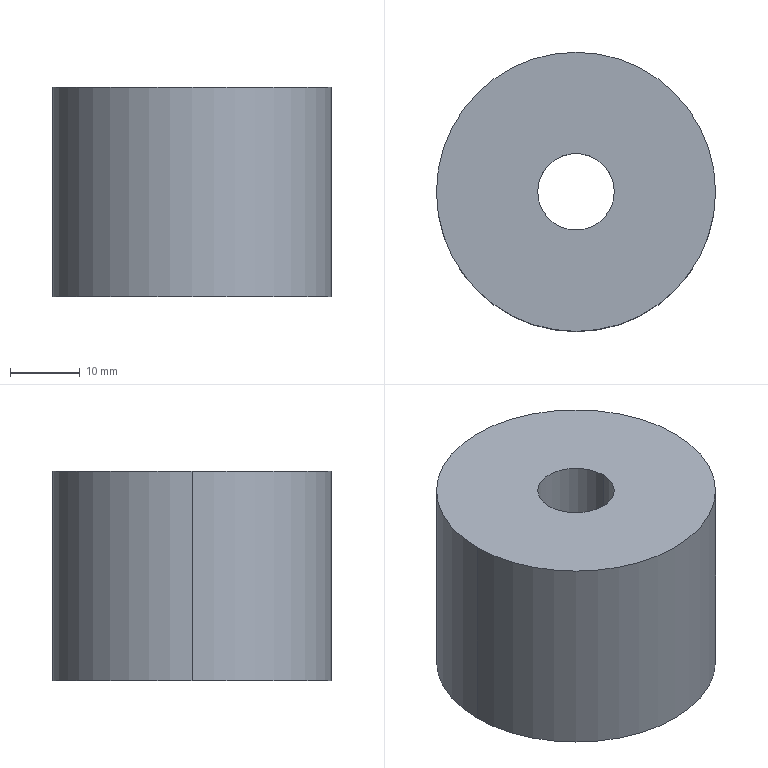Part | STEP file | X77-03029 | 1 solid | 9 faces | box 40 x 40 x 30 mm | volume 33094 mm3 | cylinder 6 | plane 3 | commonest cylinder face diameters 11 x2 18 x2 40 x2
STEP:
#1=CARTESIAN_POINT('',(9.,0.,11.));
#2=VERTEX_POINT('',#1);
#3=CARTESIAN_POINT('',(-9.,0.,11.));
#4=VERTEX_POINT('',#3);
#5=CARTESIAN_POINT('',(0.,0.,11.));
#6=DIRECTION('',(0.,0.,-1.));
#7=DIRECTION('',(-1.,0.,0.));
#8=AXIS2_PLACEMENT_3D('',#5,#6,#7);
#9=CIRCLE('',#8,9.);
#10=EDGE_CURVE('',#2,#4,#9,.T.);
#11=ORIENTED_EDGE('',*,*,#10,.F.);
#12=CARTESIAN_POINT('',(9.,0.,0.));
#13=VERTEX_POINT('',#12);
#14=CARTESIAN_POINT('',(9.,0.,0.));
#15=DIRECTION('',(0.,0.,-1.));
#16=VECTOR('',#15,1000.);
#17=LINE('',#14,#16);
#18=EDGE_CURVE('',#2,#13,#17,.T.);
#19=ORIENTED_EDGE('',*,*,#18,.T.);
#20=CARTESIAN_POINT('',(-9.,0.,0.));
#21=VERTEX_POINT('',#20);
#22=CARTESIAN_POINT('',(0.,0.,0.));
#23=DIRECTION('',(0.,0.,-1.));
#24=DIRECTION('',(-1.,0.,0.));
#25=AXIS2_PLACEMENT_3D('',#22,#23,#24);
#26=CIRCLE('',#25,9.);
#27=EDGE_CURVE('',#13,#21,#26,.T.);
#28=ORIENTED_EDGE('',*,*,#27,.T.);
#29=CARTESIAN_POINT('',(-9.,0.,0.));
#30=DIRECTION('',(0.,0.,-1.));
#31=VECTOR('',#30,1000.);
#32=LINE('',#29,#31);
#33=EDGE_CURVE('',#4,#21,#32,.T.);
#34=ORIENTED_EDGE('',*,*,#33,.F.);
#35=EDGE_LOOP('',(#11,#19,#28,#34));
#36=FACE_OUTER_BOUND('',#35,.T.);
#37=CARTESIAN_POINT('',(0.,0.,0.));
#38=DIRECTION('',(0.,0.,-1.));
#39=DIRECTION('',(-1.,0.,0.));
#40=AXIS2_PLACEMENT_3D('',#37,#38,#39);
#41=CYLINDRICAL_SURFACE('',#40,9.);
#42=ADVANCED_FACE('',(#36),#41,.F.);
#43=CARTESIAN_POINT('',(5.5,0.,30.));
#44=VERTEX_POINT('',#43);
#45=CARTESIAN_POINT('',(-5.5,0.,30.));
#46=VERTEX_POINT('',#45);
#47=CARTESIAN_POINT('',(0.,0.,30.));
#48=DIRECTION('',(0.,0.,-1.));
#49=DIRECTION('',(-1.,0.,0.));
#50=AXIS2_PLACEMENT_3D('',#47,#48,#49);
#51=CIRCLE('',#50,5.5);
#52=EDGE_CURVE('',#44,#46,#51,.T.);
#53=ORIENTED_EDGE('',*,*,#52,.F.);
#54=CARTESIAN_POINT('',(5.5,0.,11.));
#55=VERTEX_POINT('',#54);
#56=CARTESIAN_POINT('',(5.5,0.,0.));
#57=DIRECTION('',(0.,0.,-1.));
#58=VECTOR('',#57,1000.);
#59=LINE('',#56,#58);
#60=EDGE_CURVE('',#44,#55,#59,.T.);
#61=ORIENTED_EDGE('',*,*,#60,.T.);
#62=CARTESIAN_POINT('',(-5.5,0.,11.));
#63=VERTEX_POINT('',#62);
#64=CARTESIAN_POINT('',(0.,0.,11.));
#65=DIRECTION('',(0.,0.,-1.));
#66=DIRECTION('',(-1.,0.,0.));
#67=AXIS2_PLACEMENT_3D('',#64,#65,#66);
#68=CIRCLE('',#67,5.5);
#69=EDGE_CURVE('',#55,#63,#68,.T.);
#70=ORIENTED_EDGE('',*,*,#69,.T.);
#71=CARTESIAN_POINT('',(-5.5,0.,0.));
#72=DIRECTION('',(0.,0.,-1.));
#73=VECTOR('',#72,1000.);
#74=LINE('',#71,#73);
#75=EDGE_CURVE('',#46,#63,#74,.T.);
#76=ORIENTED_EDGE('',*,*,#75,.F.);
#77=EDGE_LOOP('',(#53,#61,#70,#76));
#78=FACE_OUTER_BOUND('',#77,.T.);
#79=CARTESIAN_POINT('',(0.,0.,0.));
#80=DIRECTION('',(0.,0.,-1.));
#81=DIRECTION('',(-1.,0.,0.));
#82=AXIS2_PLACEMENT_3D('',#79,#80,#81);
#83=CYLINDRICAL_SURFACE('',#82,5.5);
#84=ADVANCED_FACE('',(#78),#83,.F.);
#85=CARTESIAN_POINT('',(20.,0.,30.));
#86=VERTEX_POINT('',#85);
#87=CARTESIAN_POINT('',(-20.,0.,30.));
#88=VERTEX_POINT('',#87);
#89=CARTESIAN_POINT('',(0.,0.,30.));
#90=DIRECTION('',(0.,0.,1.));
#91=DIRECTION('',(1.,0.,0.));
#92=AXIS2_PLACEMENT_3D('',#89,#90,#91);
#93=CIRCLE('',#92,20.);
#94=EDGE_CURVE('',#86,#88,#93,.T.);
#95=ORIENTED_EDGE('',*,*,#94,.F.);
#96=CARTESIAN_POINT('',(20.,0.,0.));
#97=VERTEX_POINT('',#96);
#98=CARTESIAN_POINT('',(20.,0.,30.));
#99=DIRECTION('',(0.,0.,-1.));
#100=VECTOR('',#99,1000.);
#101=LINE('',#98,#100);
#102=EDGE_CURVE('',#86,#97,#101,.T.);
#103=ORIENTED_EDGE('',*,*,#102,.T.);
#104=CARTESIAN_POINT('',(-20.,0.,0.));
#105=VERTEX_POINT('',#104);
#106=CARTESIAN_POINT('',(0.,0.,0.));
#107=DIRECTION('',(0.,0.,1.));
#108=DIRECTION('',(1.,0.,0.));
#109=AXIS2_PLACEMENT_3D('',#106,#107,#108);
#110=CIRCLE('',#109,20.);
#111=EDGE_CURVE('',#97,#105,#110,.T.);
#112=ORIENTED_EDGE('',*,*,#111,.T.);
#113=CARTESIAN_POINT('',(-20.,0.,30.));
#114=DIRECTION('',(0.,0.,-1.));
#115=VECTOR('',#114,1000.);
#116=LINE('',#113,#115);
#117=EDGE_CURVE('',#88,#105,#116,.T.);
#118=ORIENTED_EDGE('',*,*,#117,.F.);
#119=EDGE_LOOP('',(#95,#103,#112,#118));
#120=FACE_OUTER_BOUND('',#119,.T.);
#121=CARTESIAN_POINT('',(0.,0.,30.));
#122=DIRECTION('',(0.,0.,-1.));
#123=DIRECTION('',(-1.,0.,0.));
#124=AXIS2_PLACEMENT_3D('',#121,#122,#123);
#125=CYLINDRICAL_SURFACE('',#124,20.);
#126=ADVANCED_FACE('',(#120),#125,.T.);
#127=ORIENTED_EDGE('',*,*,#102,.F.);
#128=CARTESIAN_POINT('',(0.,0.,30.));
#129=DIRECTION('',(0.,0.,1.));
#130=DIRECTION('',(1.,0.,0.));
#131=AXIS2_PLACEMENT_3D('',#128,#129,#130);
#132=CIRCLE('',#131,20.);
#133=EDGE_CURVE('',#88,#86,#132,.T.);
#134=ORIENTED_EDGE('',*,*,#133,.F.);
#135=ORIENTED_EDGE('',*,*,#117,.T.);
#136=CARTESIAN_POINT('',(0.,0.,0.));
#137=DIRECTION('',(0.,0.,1.));
#138=DIRECTION('',(1.,0.,0.));
#139=AXIS2_PLACEMENT_3D('',#136,#137,#138);
#140=CIRCLE('',#139,20.);
#141=EDGE_CURVE('',#105,#97,#140,.T.);
#142=ORIENTED_EDGE('',*,*,#141,.T.);
#143=EDGE_LOOP('',(#127,#134,#135,#142));
#144=FACE_OUTER_BOUND('',#143,.T.);
#145=CARTESIAN_POINT('',(0.,0.,30.));
#146=DIRECTION('',(0.,0.,-1.));
#147=DIRECTION('',(-1.,0.,0.));
#148=AXIS2_PLACEMENT_3D('',#145,#146,#147);
#149=CYLINDRICAL_SURFACE('',#148,20.);
#150=ADVANCED_FACE('',(#144),#149,.T.);
#151=CARTESIAN_POINT('',(0.,0.,30.));
#152=DIRECTION('',(0.,0.,-1.));
#153=DIRECTION('',(-1.,0.,0.));
#154=AXIS2_PLACEMENT_3D('',#151,#152,#153);
#155=CIRCLE('',#154,5.5);
#156=EDGE_CURVE('',#46,#44,#155,.T.);
#157=ORIENTED_EDGE('',*,*,#156,.T.);
#158=ORIENTED_EDGE('',*,*,#52,.T.);
#159=EDGE_LOOP('',(#157,#158));
#160=FACE_BOUND('',#159,.T.);
#161=ORIENTED_EDGE('',*,*,#133,.T.);
#162=ORIENTED_EDGE('',*,*,#94,.T.);
#163=EDGE_LOOP('',(#161,#162));
#164=FACE_OUTER_BOUND('',#163,.T.);
#165=CARTESIAN_POINT('',(0.,0.,30.));
#166=DIRECTION('',(0.,0.,1.));
#167=DIRECTION('',(1.,0.,0.));
#168=AXIS2_PLACEMENT_3D('',#165,#166,#167);
#169=PLANE('',#168);
#170=ADVANCED_FACE('',(#160,#164),#169,.T.);
#171=CARTESIAN_POINT('',(0.,0.,0.));
#172=DIRECTION('',(0.,0.,-1.));
#173=DIRECTION('',(-1.,0.,0.));
#174=AXIS2_PLACEMENT_3D('',#171,#172,#173);
#175=CIRCLE('',#174,9.);
#176=EDGE_CURVE('',#21,#13,#175,.T.);
#177=ORIENTED_EDGE('',*,*,#176,.F.);
#178=ORIENTED_EDGE('',*,*,#27,.F.);
#179=EDGE_LOOP('',(#177,#178));
#180=FACE_BOUND('',#179,.T.);
#181=ORIENTED_EDGE('',*,*,#141,.F.);
#182=ORIENTED_EDGE('',*,*,#111,.F.);
#183=EDGE_LOOP('',(#181,#182));
#184=FACE_OUTER_BOUND('',#183,.T.);
#185=CARTESIAN_POINT('',(0.,0.,0.));
#186=DIRECTION('',(0.,0.,1.));
#187=DIRECTION('',(1.,0.,0.));
#188=AXIS2_PLACEMENT_3D('',#185,#186,#187);
#189=PLANE('',#188);
#190=ADVANCED_FACE('',(#180,#184),#189,.F.);
#191=ORIENTED_EDGE('',*,*,#60,.F.);
#192=ORIENTED_EDGE('',*,*,#156,.F.);
#193=ORIENTED_EDGE('',*,*,#75,.T.);
#194=CARTESIAN_POINT('',(0.,0.,11.));
#195=DIRECTION('',(0.,0.,-1.));
#196=DIRECTION('',(-1.,0.,0.));
#197=AXIS2_PLACEMENT_3D('',#194,#195,#196);
#198=CIRCLE('',#197,5.5);
#199=EDGE_CURVE('',#63,#55,#198,.T.);
#200=ORIENTED_EDGE('',*,*,#199,.T.);
#201=EDGE_LOOP('',(#191,#192,#193,#200));
#202=FACE_OUTER_BOUND('',#201,.T.);
#203=CARTESIAN_POINT('',(0.,0.,0.));
#204=DIRECTION('',(0.,0.,-1.));
#205=DIRECTION('',(-1.,0.,0.));
#206=AXIS2_PLACEMENT_3D('',#203,#204,#205);
#207=CYLINDRICAL_SURFACE('',#206,5.5);
#208=ADVANCED_FACE('',(#202),#207,.F.);
#209=ORIENTED_EDGE('',*,*,#199,.F.);
#210=ORIENTED_EDGE('',*,*,#69,.F.);
#211=EDGE_LOOP('',(#209,#210));
#212=FACE_BOUND('',#211,.T.);
#213=CARTESIAN_POINT('',(0.,0.,11.));
#214=DIRECTION('',(0.,0.,-1.));
#215=DIRECTION('',(-1.,0.,0.));
#216=AXIS2_PLACEMENT_3D('',#213,#214,#215);
#217=CIRCLE('',#216,9.);
#218=EDGE_CURVE('',#4,#2,#217,.T.);
#219=ORIENTED_EDGE('',*,*,#218,.T.);
#220=ORIENTED_EDGE('',*,*,#10,.T.);
#221=EDGE_LOOP('',(#219,#220));
#222=FACE_OUTER_BOUND('',#221,.T.);
#223=CARTESIAN_POINT('',(5.5,0.,11.));
#224=DIRECTION('',(0.,0.,1.));
#225=DIRECTION('',(1.,0.,0.));
#226=AXIS2_PLACEMENT_3D('',#223,#224,#225);
#227=PLANE('',#226);
#228=ADVANCED_FACE('',(#212,#222),#227,.F.);
#229=ORIENTED_EDGE('',*,*,#18,.F.);
#230=ORIENTED_EDGE('',*,*,#218,.F.);
#231=ORIENTED_EDGE('',*,*,#33,.T.);
#232=ORIENTED_EDGE('',*,*,#176,.T.);
#233=EDGE_LOOP('',(#229,#230,#231,#232));
#234=FACE_OUTER_BOUND('',#233,.T.);
#235=CARTESIAN_POINT('',(0.,0.,0.));
#236=DIRECTION('',(0.,0.,-1.));
#237=DIRECTION('',(-1.,0.,0.));
#238=AXIS2_PLACEMENT_3D('',#235,#236,#237);
#239=CYLINDRICAL_SURFACE('',#238,9.);
#240=ADVANCED_FACE('',(#234),#239,.F.);
#241=CLOSED_SHELL('',(#42,#84,#126,#150,#170,#190,#208,#228,#240));
#242=MANIFOLD_SOLID_BREP('',#241);
#243=CARTESIAN_POINT('',(0.,0.,0.));
#244=DIRECTION('',(0.,0.,1.));
#245=DIRECTION('',(1.,0.,0.));
#246=AXIS2_PLACEMENT_3D('',#243,#244,#245);
#247=(LENGTH_UNIT()NAMED_UNIT(*)SI_UNIT(.MILLI.,.METRE.));
#248=UNCERTAINTY_MEASURE_WITH_UNIT(LENGTH_MEASURE(0.00001),#247,'','');
#249=(NAMED_UNIT(*)PLANE_ANGLE_UNIT()SI_UNIT($,.RADIAN.));
#250=(NAMED_UNIT(*)SI_UNIT($,.STERADIAN.)SOLID_ANGLE_UNIT());
#251=(GEOMETRIC_REPRESENTATION_CONTEXT(3)GLOBAL_UNCERTAINTY_ASSIGNED_CONTEXT((#248))GLOBAL_UNIT_ASSIGNED_CONTEXT((#247,#249,#250))REPRESENTATION_CONTEXT('',''));
#252=ADVANCED_BREP_SHAPE_REPRESENTATION('',(#242,#246),#251);